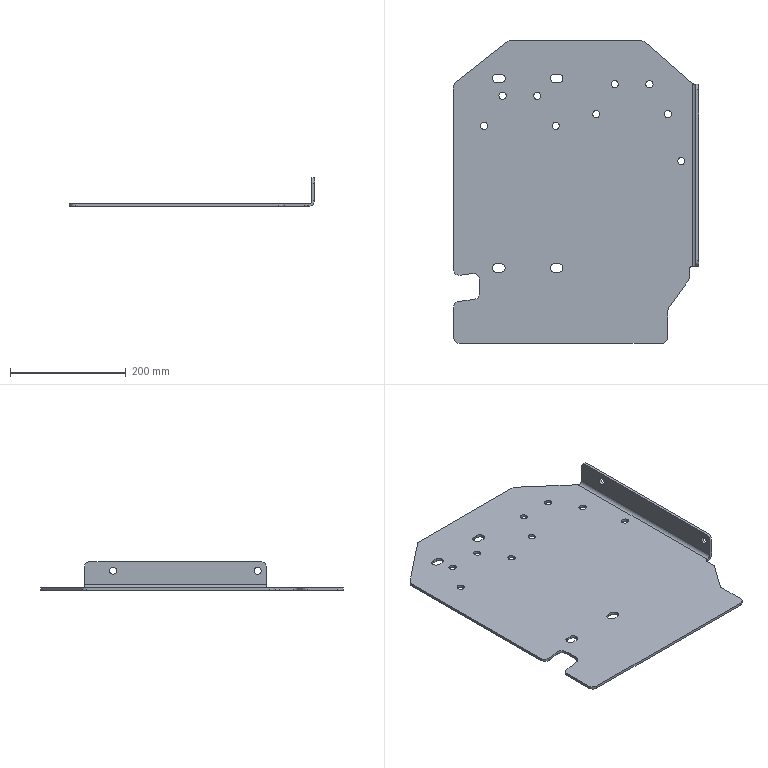Part | SolidWorks | features EdgeFlange 1, Fillet 1, FlatPattern 1, ICE 1, SMBaseFlange 1, SheetMetal 1 | 1 solid | 84 faces | box 424 x 523 x 50 mm | volume 979518 mm3 | cylinder 51 | plane 33 | commonest cylinder face diameters 12.5 x22 20 x14 15 x12 6 x1 12 x1 21 x1